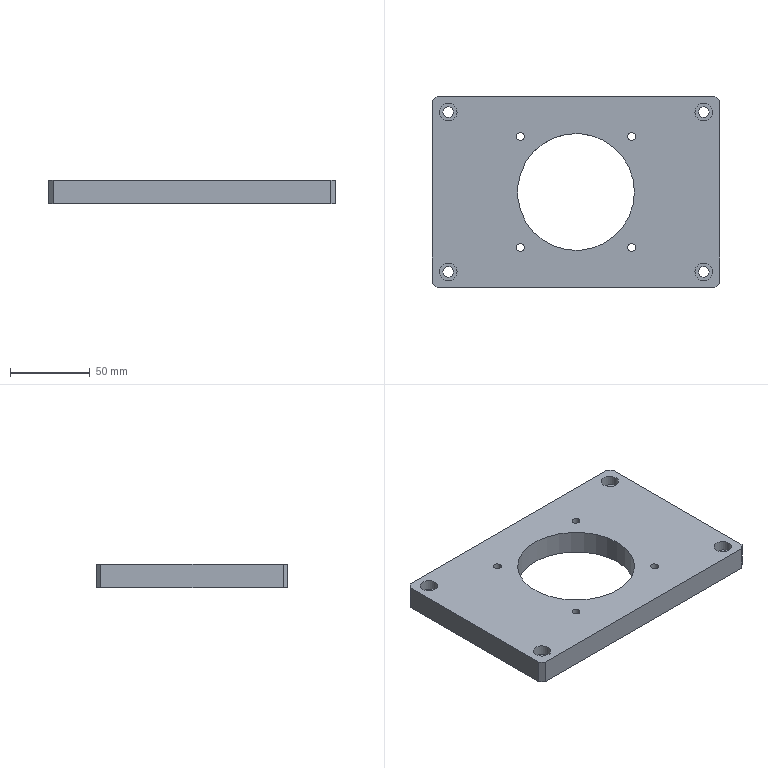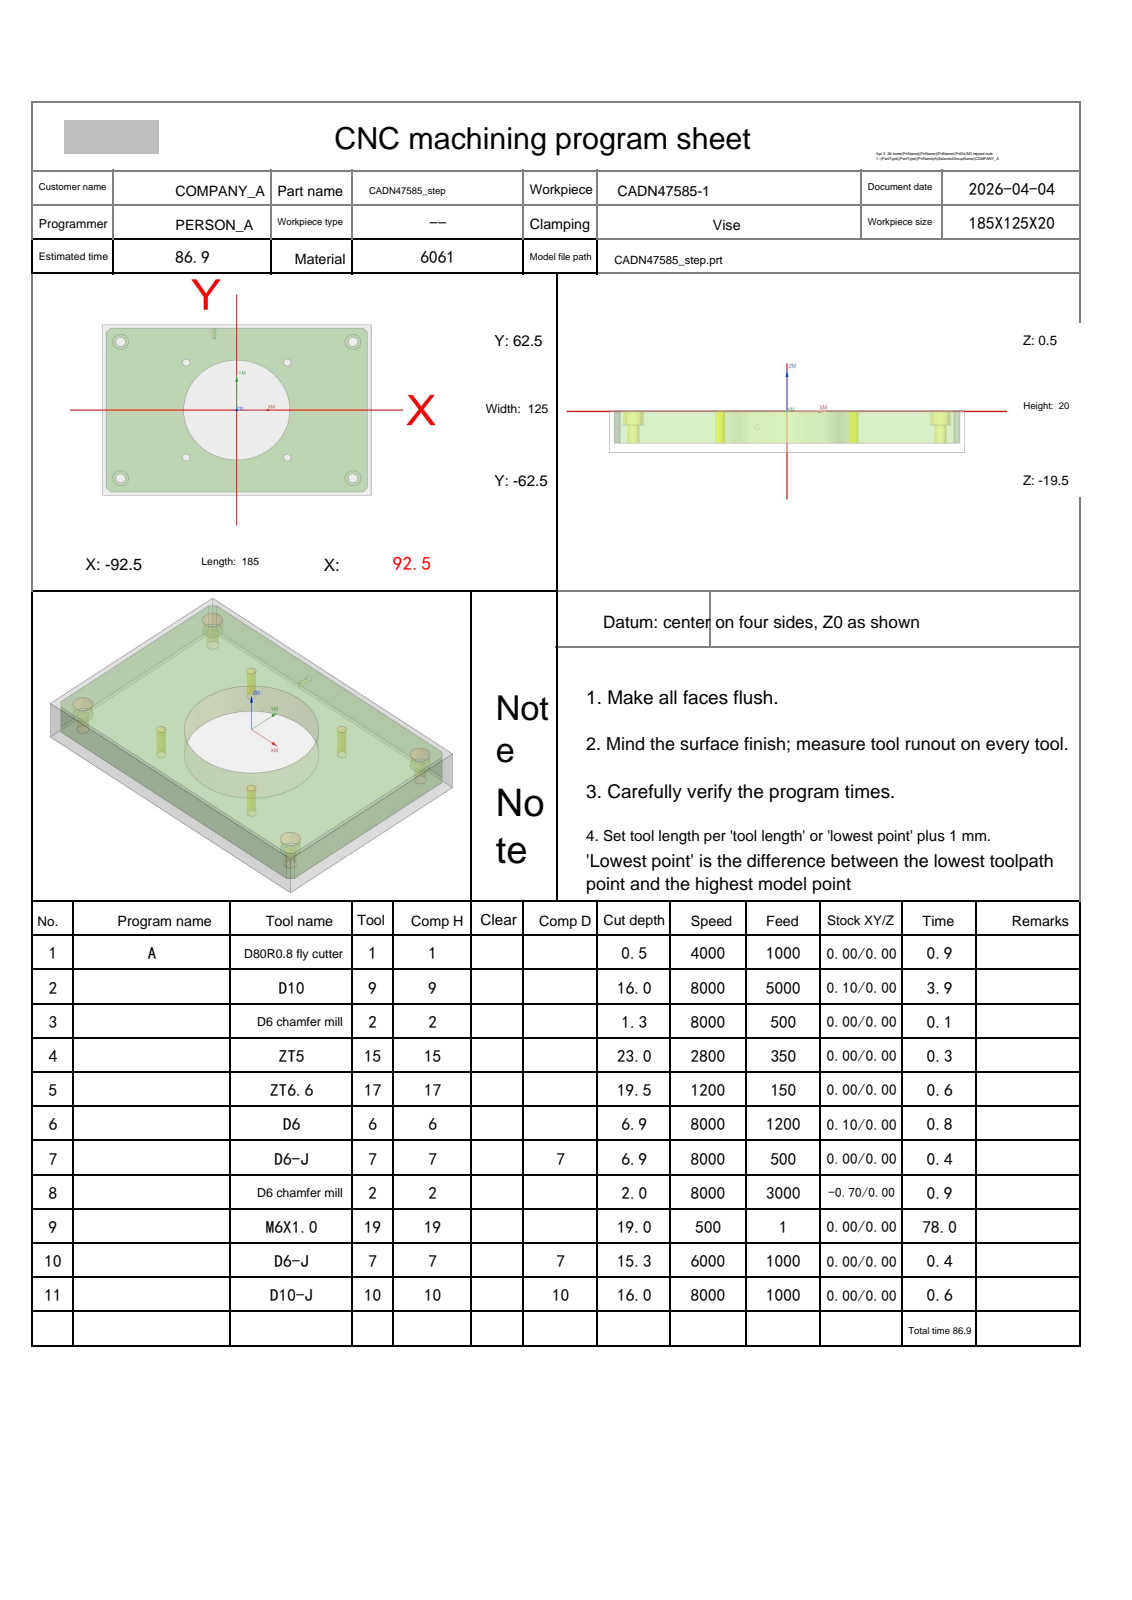NC program | NX | posted by the shop | part box 180 x 120 x 15 mm
Whole program:
%
O0001
(Machine time: 163.22 MIN)
(===Total Tool:9===)
(T1=D80R0.8 fly cutter D=80.  R=0.8  D-  H01 Z=0.    )
(T9=D10     D=10.  R=0.   D-  H09 Z=-15.5 )
(T2=D6 chamfer mill   D=6.   R=0.   D-  H02 Z=-1.5  )
(T15=ZT5    D=5.   DR_a=118 D-  H15 Z=-22.5 )
(T17=ZT6.6  D=6.6  DR_a=118 D-  H17 Z=-18.98)
(T6=D6      D=6.   R=0.   D-  H06 Z=-6.4  )
(T7=D6-J    D=6.   R=0.   D7  H07 Z=-14.8 )
(T19=M6X1.0 D=5.   DR_a=180 D-  H19 Z=-18.5 )
(T10=D10-J  D=10.  R=0.   D10 H10 Z=-15.5 )
G80 G90 G17 G49 G40
G91 G28 Z0
M01
N1 T01 M06
(D80R0.8 fly cutter  D=80. R=0.8 H=01 ce=0.00 di=0.00)
G00 G90 G54 X-135. Y50. M03 S4000
G43 H01 Z20.
M08
Z2.
G01 Z0.0 F1000.
X-130.
X130.
Y0.0
X-130.
Y-50.
X130.
X135.
Z2.
G00 Z20.
G91 G28 Z0.0
M05
M09
G91 G28 Z0.0
M01
N2 T09 M06
(D10  D=10. R=0. H=09 ce=0.10 di=0.00)
G00 G90 G54 X0.0 Y65.1 M03 S8000
G43 H09 Z20.
M08
Z.5
G01 X87. Z.389 F5000.
G02 X90.606 Y63.606 Z.384 I0.0 J-5.1
G01 X93.606 Y60.606 Z.378
G02 X95.1 Y57. Z.373 I-3.606 J-3.606
G01 Y-57. Z.227
G02 X93.606 Y-60.606 Z.222 I-5.1 J0.0
G01 X90.606 Y-63.606 Z.216
G02 X87. Y-65.1 Z.211 I-3.606 J3.606
G01 X-87. Z-.011
G02 X-90.606 Y-63.606 Z-.016 I0.0 J5.1
G01 X-93.606 Y-60.606 Z-.022
G02 X-95.1 Y-57. Z-.027 I3.606 J3.606
G01 Y57. Z-.173
G02 X-93.606 Y60.606 Z-.178 I5.1 J0.0
G01 X-90.606 Y63.606 Z-.184
G02 X-87. Y65.1 Z-.189 I3.606 J-3.606
G01 X87. Z-.411
G02 X90.606 Y63.606 Z-.416 I0.0 J-5.1
G01 X93.606 Y60.606 Z-.422
G02 X95.1 Y57. Z-.427 I-3.606 J-3.606
G01 Y-57. Z-.573
G02 X93.606 Y-60.606 Z-.578 I-5.1 J0.0
G01 X90.606 Y-63.606 Z-.584
G02 X87. Y-65.1 Z-.589 I-3.606 J3.606
G01 X-87. Z-.811
G02 X-90.606 Y-63.606 Z-.816 I0.0 J5.1
G01 X-93.606 Y-60.606 Z-.822
G02 X-95.1 Y-57. Z-.827 I3.606 J3.606
G01 Y57. Z-.973
G02 X-93.606 Y60.606 Z-.978 I5.1 J0.0
G01 X-90.606 Y63.606 Z-.984
G02 X-87. Y65.1 Z-.989 I3.606 J-3.606
G01 X87. Z-1.211
G02 X90.606 Y63.606 Z-1.216 I0.0 J-5.1
G01 X93.606 Y60.606 Z-1.222
G02 X95.1 Y57. Z-1.227 I-3.606 J-3.606
G01 Y-57. Z-1.373
G02 X93.606 Y-60.606 Z-1.378 I-5.1 J0.0
G01 X90.606 Y-63.606 Z-1.384
G02 X87. Y-65.1 Z-1.389 I-3.606 J3.606
G01 X-87. Z-1.611
G02 X-90.606 Y-63.606 Z-1.616 I0.0 J5.1
G01 X-93.606 Y-60.606 Z-1.622
G02 X-95.1 Y-57. Z-1.627 I3.606 J3.606
G01 Y57. Z-1.773
G02 X-93.606 Y60.606 Z-1.778 I5.1 J0.0
G01 X-90.606 Y63.606 Z-1.784
G02 X-87. Y65.1 Z-1.789 I3.606 J-3.606
G01 X87. Z-2.011
G02 X90.606 Y63.606 Z-2.016 I0.0 J-5.1
G01 X93.606 Y60.606 Z-2.022
G02 X95.1 Y57. Z-2.027 I-3.606 J-3.606
G01 Y-57. Z-2.173
G02 X93.606 Y-60.606 Z-2.178 I-5.1 J0.0
G01 X90.606 Y-63.606 Z-2.184
G02 X87. Y-65.1 Z-2.189 I-3.606 J3.606
G01 X-87. Z-2.411
G02 X-90.606 Y-63.606 Z-2.416 I0.0 J5.1
G01 X-93.606 Y-60.606 Z-2.422
G02 X-95.1 Y-57. Z-2.427 I3.606 J3.606
G01 Y57. Z-2.573
G02 X-93.606 Y60.606 Z-2.578 I5.1 J0.0
G01 X-90.606 Y63.606 Z-2.584
G02 X-87. Y65.1 Z-2.589 I3.606 J-3.606
G01 X87. Z-2.811
G02 X90.606 Y63.606 Z-2.816 I0.0 J-5.1
G01 X93.606 Y60.606 Z-2.822
G02 X95.1 Y57. Z-2.827 I-3.606 J-3.606
G01 Y-57. Z-2.973
G02 X93.606 Y-60.606 Z-2.978 I-5.1 J0.0
G01 X90.606 Y-63.606 Z-2.984
G02 X87. Y-65.1 Z-2.989 I-3.606 J3.606
G01 X-87. Z-3.211
G02 X-90.606 Y-63.606 Z-3.216 I0.0 J5.1
G01 X-93.606 Y-60.606 Z-3.222
G02 X-95.1 Y-57. Z-3.227 I3.606 J3.606
G01 Y57. Z-3.373
G02 X-93.606 Y60.606 Z-3.378 I5.1 J0.0
G01 X-90.606 Y63.606 Z-3.384
G02 X-87. Y65.1 Z-3.389 I3.606 J-3.606
G01 X87. Z-3.611
G02 X90.606 Y63.606 Z-3.616 I0.0 J-5.1
G01 X93.606 Y60.606 Z-3.622
G02 X95.1 Y57. Z-3.627 I-3.606 J-3.606
G01 Y-57. Z-3.773
G02 X93.606 Y-60.606 Z-3.778 I-5.1 J0.0
G01 X90.606 Y-63.606 Z-3.784
G02 X87. Y-65.1 Z-3.789 I-3.606 J3.606
G01 X-87. Z-4.011
G02 X-90.606 Y-63.606 Z-4.016 I0.0 J5.1
G01 X-93.606 Y-60.606 Z-4.022
G02 X-95.1 Y-57. Z-4.027 I3.606 J3.606
G01 Y57. Z-4.173
G02 X-93.606 Y60.606 Z-4.178 I5.1 J0.0
G01 X-90.606 Y63.606 Z-4.184
G02 X-87. Y65.1 Z-4.189 I3.606 J-3.606
G01 X87. Z-4.411
G02 X90.606 Y63.606 Z-4.416 I0.0 J-5.1
G01 X93.606 Y60.606 Z-4.422
G02 X95.1 Y57. Z-4.427 I-3.606 J-3.606
G01 Y-57. Z-4.573
G02 X93.606 Y-60.606 Z-4.578 I-5.1 J0.0
G01 X90.606 Y-63.606 Z-4.584
G02 X87. Y-65.1 Z-4.589 I-3.606 J3.606
G01 X-87. Z-4.811
G02 X-90.606 Y-63.606 Z-4.816 I0.0 J5.1
G01 X-93.606 Y-60.606 Z-4.822
G02 X-95.1 Y-57. Z-4.827 I3.606 J3.606
G01 Y57. Z-4.973
G02 X-93.606 Y60.606 Z-4.978 I5.1 J0.0
G01 X-90.606 Y63.606 Z-4.984
G02 X-87. Y65.1 Z-4.989 I3.606 J-3.606
G01 X87. Z-5.211
G02 X90.606 Y63.606 Z-5.216 I0.0 J-5.1
G01 X93.606 Y60.606 Z-5.222
G02 X95.1 Y57. Z-5.227 I-3.606 J-3.606
G01 Y-57. Z-5.373
G02 X93.606 Y-60.606 Z-5.378 I-5.1 J0.0
G01 X90.606 Y-63.606 Z-5.384
G02 X87. Y-65.1 Z-5.389 I-3.606 J3.606
G01 X-87. Z-5.611
G02 X-90.606 Y-63.606 Z-5.616 I0.0 J5.1
G01 X-93.606 Y-60.606 Z-5.622
G02 X-95.1 Y-57. Z-5.627 I3.606 J3.606
G01 Y57. Z-5.773
G02 X-93.606 Y60.606 Z-5.778 I5.1 J0.0
G01 X-90.606 Y63.606 Z-5.784
G02 X-87. Y65.1 Z-5.789 I3.606 J-3.606
G01 X87. Z-6.011
G02 X90.606 Y63.606 Z-6.016 I0.0 J-5.1
G01 X93.606 Y60.606 Z-6.022
G02 X95.1 Y57. Z-6.027 I-3.606 J-3.606
G01 Y-57. Z-6.173
G02 X93.606 Y-60.606 Z-6.178 I-5.1 J0.0
G01 X90.606 Y-63.606 Z-6.184
G02 X87. Y-65.1 Z-6.189 I-3.606 J3.606
G01 X-87. Z-6.411
G02 X-90.606 Y-63.606 Z-6.416 I0.0 J5.1
G01 X-93.606 Y-60.606 Z-6.422
G02 X-95.1 Y-57. Z-6.427 I3.606 J3.606
G01 Y57. Z-6.573
G02 X-93.606 Y60.606 Z-6.578 I5.1 J0.0
G01 X-90.606 Y63.606 Z-6.584
G02 X-87. Y65.1 Z-6.589 I3.606 J-3.606
G01 X87. Z-6.811
G02 X90.606 Y63.606 Z-6.816 I0.0 J-5.1
G01 X93.606 Y60.606 Z-6.822
G02 X95.1 Y57. Z-6.827 I-3.606 J-3.606
G01 Y-57. Z-6.973
G02 X93.606 Y-60.606 Z-6.978 I-5.1 J0.0
G01 X90.606 Y-63.606 Z-6.984
G02 X87. Y-65.1 Z-6.989 I-3.606 J3.606
G01 X-87. Z-7.211
G02 X-90.606 Y-63.606 Z-7.216 I0.0 J5.1
G01 X-93.606 Y-60.606 Z-7.222
G02 X-95.1 Y-57. Z-7.227 I3.606 J3.606
G01 Y57. Z-7.373
G02 X-93.606 Y60.606 Z-7.378 I5.1 J0.0
G01 X-90.606 Y63.606 Z-7.384
G02 X-87. Y65.1 Z-7.389 I3.606 J-3.606
G01 X87. Z-7.611
G02 X90.606 Y63.606 Z-7.616 I0.0 J-5.1
G01 X93.606 Y60.606 Z-7.622
G02 X95.1 Y57. Z-7.627 I-3.606 J-3.606
G01 Y-57. Z-7.773
G02 X93.606 Y-60.606 Z-7.778 I-5.1 J0.0
G01 X90.606 Y-63.606 Z-7.784
G02 X87. Y-65.1 Z-7.789 I-3.606 J3.606
G01 X-87. Z-8.011
G02 X-90.606 Y-63.606 Z-8.016 I0.0 J5.1
G01 X-93.606 Y-60.606 Z-8.022
G02 X-95.1 Y-57. Z-8.027 I3.606 J3.606
G01 Y57. Z-8.173
G02 X-93.606 Y60.606 Z-8.178 I5.1 J0.0
G01 X-90.606 Y63.606 Z-8.184
G02 X-87. Y65.1 Z-8.189 I3.606 J-3.606
G01 X87. Z-8.411
G02 X90.606 Y63.606 Z-8.416 I0.0 J-5.1
G01 X93.606 Y60.606 Z-8.422
G02 X95.1 Y57. Z-8.427 I-3.606 J-3.606
G01 Y-57. Z-8.573
G02 X93.606 Y-60.606 Z-8.578 I-5.1 J0.0
G01 X90.606 Y-63.606 Z-8.584
G02 X87. Y-65.1 Z-8.589 I-3.606 J3.606
G01 X-87. Z-8.811
G02 X-90.606 Y-63.606 Z-8.816 I0.0 J5.1
G01 X-93.606 Y-60.606 Z-8.822
G02 X-95.1 Y-57. Z-8.827 I3.606 J3.606
G01 Y57. Z-8.973
G02 X-93.606 Y60.606 Z-8.978 I5.1 J0.0
G01 X-90.606 Y63.606 Z-8.984
G02 X-87. Y65.1 Z-8.989 I3.606 J-3.606
G01 X87. Z-9.211
G02 X90.606 Y63.606 Z-9.216 I0.0 J-5.1
G01 X93.606 Y60.606 Z-9.222
G02 X95.1 Y57. Z-9.227 I-3.606 J-3.606
G01 Y-57. Z-9.373
G02 X93.606 Y-60.606 Z-9.378 I-5.1 J0.0
G01 X90.606 Y-63.606 Z-9.384
G02 X87. Y-65.1 Z-9.389 I-3.606 J3.606
G01 X-87. Z-9.611
G02 X-90.606 Y-63.606 Z-9.616 I0.0 J5.1
G01 X-93.606 Y-60.606 Z-9.622
G02 X-95.1 Y-57. Z-9.627 I3.606 J3.606
G01 Y57. Z-9.773
G02 X-93.606 Y60.606 Z-9.778 I5.1 J0.0
G01 X-90.606 Y63.606 Z-9.784
G02 X-87. Y65.1 Z-9.789 I3.606 J-3.606
G01 X87. Z-10.011
G02 X90.606 Y63.606 Z-10.016 I0.0 J-5.1
G01 X93.606 Y60.606 Z-10.022
G02 X95.1 Y57. Z-10.027 I-3.606 J-3.606
G01 Y-57. Z-10.173
G02 X93.606 Y-60.606 Z-10.178 I-5.1 J0.0
G01 X90.606 Y-63.606 Z-10.184
G02 X87. Y-65.1 Z-10.189 I-3.606 J3.606
G01 X-87. Z-10.411
G02 X-90.606 Y-63.606 Z-10.416 I0.0 J5.1
G01 X-93.606 Y-60.606 Z-10.422
G02 X-95.1 Y-57. Z-10.427 I3.606 J3.606
G01 Y57. Z-10.573
G02 X-93.606 Y60.606 Z-10.578 I5.1 J0.0
G01 X-90.606 Y63.606 Z-10.584
G02 X-87. Y65.1 Z-10.589 I3.606 J-3.606
G01 X87. Z-10.811
G02 X90.606 Y63.606 Z-10.816 I0.0 J-5.1
G01 X93.606 Y60.606 Z-10.822
G02 X95.1 Y57. Z-10.827 I-3.606 J-3.606
G01 Y-57. Z-10.973
G02 X93.606 Y-60.606 Z-10.978 I-5.1 J0.0
G01 X90.606 Y-63.606 Z-10.984
G02 X87. Y-65.1 Z-10.989 I-3.606 J3.606
G01 X-87. Z-11.211
G02 X-90.606 Y-63.606 Z-11.216 I0.0 J5.1
G01 X-93.606 Y-60.606 Z-11.222
G02 X-95.1 Y-57. Z-11.227 I3.606 J3.606
G01 Y57. Z-11.373
G02 X-93.606 Y60.606 Z-11.378 I5.1 J0.0
G01 X-90.606 Y63.606 Z-11.384
G02 X-87. Y65.1 Z-11.389 I3.606 J-3.606
G01 X87. Z-11.611
G02 X90.606 Y63.606 Z-11.616 I0.0 J-5.1
G01 X93.606 Y60.606 Z-11.622
G02 X95.1 Y57. Z-11.627 I-3.606 J-3.606
G01 Y-57. Z-11.773
G02 X93.606 Y-60.606 Z-11.778 I-5.1 J0.0
G01 X90.606 Y-63.606 Z-11.784
G02 X87. Y-65.1 Z-11.789 I-3.606 J3.606
G01 X-87. Z-12.011
G02 X-90.606 Y-63.606 Z-12.016 I0.0 J5.1
G01 X-93.606 Y-60.606 Z-12.022
G02 X-95.1 Y-57. Z-12.027 I3.606 J3.606
G01 Y57. Z-12.173
G02 X-93.606 Y60.606 Z-12.178 I5.1 J0.0
G01 X-90.606 Y63.606 Z-12.184
G02 X-87. Y65.1 Z-12.189 I3.606 J-3.606
G01 X87. Z-12.411
G02 X90.606 Y63.606 Z-12.416 I0.0 J-5.1
G01 X93.606 Y60.606 Z-12.422
G02 X95.1 Y57. Z-12.427 I-3.606 J-3.606
G01 Y-57. Z-12.573
G02 X93.606 Y-60.606 Z-12.578 I-5.1 J0.0
G01 X90.606 Y-63.606 Z-12.584
G02 X87. Y-65.1 Z-12.589 I-3.606 J3.606
G01 X-87. Z-12.811
G02 X-90.606 Y-63.606 Z-12.816 I0.0 J5.1
G01 X-93.606 Y-60.606 Z-12.822
G02 X-95.1 Y-57. Z-12.827 I3.606 J3.606
G01 Y57. Z-12.973
G02 X-93.606 Y60.606 Z-12.978 I5.1 J0.0
G01 X-90.606 Y63.606 Z-12.984
G02 X-87. Y65.1 Z-12.989 I3.606 J-3.606
G01 X87. Z-13.211
G02 X90.606 Y63.606 Z-13.216 I0.0 J-5.1
G01 X93.606 Y60.606 Z-13.222
G02 X95.1 Y57. Z-13.227 I-3.606 J-3.606
G01 Y-57. Z-13.373
G02 X93.606 Y-60.606 Z-13.378 I-5.1 J0.0
G01 X90.606 Y-63.606 Z-13.384
G02 X87. Y-65.1 Z-13.389 I-3.606 J3.606
G01 X-87. Z-13.611
G02 X-90.606 Y-63.606 Z-13.616 I0.0 J5.1
G01 X-93.606 Y-60.606 Z-13.622
G02 X-95.1 Y-57. Z-13.627 I3.606 J3.606
G01 Y57. Z-13.773
G02 X-93.606 Y60.606 Z-13.778 I5.1 J0.0
G01 X-90.606 Y63.606 Z-13.784
G02 X-87. Y65.1 Z-13.789 I3.606 J-3.606
G01 X87. Z-14.011
G02 X90.606 Y63.606 Z-14.016 I0.0 J-5.1
G01 X93.606 Y60.606 Z-14.022
G02 X95.1 Y57. Z-14.027 I-3.606 J-3.606
G01 Y-57. Z-14.173
G02 X93.606 Y-60.606 Z-14.178 I-5.1 J0.0
G01 X90.606 Y-63.606 Z-14.184
G02 X87. Y-65.1 Z-14.189 I-3.606 J3.606
G01 X-87. Z-14.411
G02 X-90.606 Y-63.606 Z-14.416 I0.0 J5.1
G01 X-93.606 Y-60.606 Z-14.422
G02 X-95.1 Y-57. Z-14.427 I3.606 J3.606
G01 Y57. Z-14.573
G02 X-93.606 Y60.606 Z-14.578 I5.1 J0.0
G01 X-90.606 Y63.606 Z-14.584
G02 X-87. Y65.1 Z-14.589 I3.606 J-3.606
G01 X87. Z-14.811
G02 X90.606 Y63.606 Z-14.816 I0.0 J-5.1
G01 X93.606 Y60.606 Z-14.822
G02 X95.1 Y57. Z-14.827 I-3.606 J-3.606
G01 Y-57. Z-14.973
G02 X93.606 Y-60.606 Z-14.978 I-5.1 J0.0
G01 X90.606 Y-63.606 Z-14.984
G02 X87. Y-65.1 Z-14.989 I-3.606 J3.606
G01 X-87. Z-15.211
G02 X-90.606 Y-63.606 Z-15.216 I0.0 J5.1
G01 X-93.606 Y-60.606 Z-15.222
G02 X-95.1 Y-57. Z-15.227 I3.606 J3.606
G01 Y57. Z-15.373
G02 X-93.606 Y60.606 Z-15.378 I5.1 J0.0
G01 X-90.606 Y63.606 Z-15.384
G02 X-87. Y65.1 Z-15.389 I3.606 J-3.606
G01 X0.0 Z-15.5
X87.
G02 X90.606 Y63.606 I0.0 J-5.1
G01 X93.606 Y60.606
G02 X95.1 Y57. I-3.606 J-3.606
G01 Y-57.
G02 X93.606 Y-60.606 I-5.1 J0.0
G01 X90.606 Y-63.606
G02 X87. Y-65.1 I-3.606 J3.606
G01 X-87.
G02 X-90.606 Y-63.606 I0.0 J5.1
G01 X-93.606 Y-60.606
G02 X-95.1 Y-57. I3.606 J3.606
G01 Y57.
G02 X-93.606 Y60.606 I5.1 J0.0
G01 X-90.606 Y63.606
G02 X-87. Y65.1 I3.606 J-3.606
G01 X0.0
X.5
Z-14.5
G00 Z20.
G00 G90 X17.938 Y25.912 M03 S8000
Z20.
Z1.
G01 X15.119 Y27.669 Z.826 F4000.
X11.87 Y29.21 Z.637
X8.467 Y30.372 Z.449
X4.953 Y31.139 Z.261
X1.375 Y31.5 Z.072
X0.0 Z0.0
G03 X-31.5 Y0.0 Z-.148 I0.0 J-31.5
X0.0 Y-31.5 Z-.296 I31.5 J0.0
X31.5 Y0.0 Z-.444 I0.0 J31.5
X0.0 Y31.5 Z-.592 I-31.5 J0.0
X-31.5 Y0.0 Z-.74 I0.0 J-31.5
X0.0 Y-31.5 Z-.888 I31.5 J0.0
X31.5 Y0.0 Z-1.036 I0.0 J31.5
X0.0 Y31.5 Z-1.184 I-31.5 J0.0
X-31.5 Y0.0 Z-1.332 I0.0 J-31.5
X0.0 Y-31.5 Z-1.48 I31.5 J0.0
X31.5 Y0.0 Z-1.628 I0.0 J31.5
X0.0 Y31.5 Z-1.776 I-31.5 J0.0
X-31.5 Y0.0 Z-1.924 I0.0 J-31.5
X0.0 Y-31.5 Z-2.072 I31.5 J0.0
X31.5 Y0.0 Z-2.22 I0.0 J31.5
X0.0 Y31.5 Z-2.368 I-31.5 J0.0
X-31.5 Y0.0 Z-2.516 I0.0 J-31.5
X0.0 Y-31.5 Z-2.664 I31.5 J0.0
X31.5 Y0.0 Z-2.812 I0.0 J31.5
X0.0 Y31.5 Z-2.96 I-31.5 J0.0
X-31.5 Y0.0 Z-3.108 I0.0 J-31.5
X0.0 Y-31.5 Z-3.256 I31.5 J0.0
X31.5 Y0.0 Z-3.404 I0.0 J31.5
X0.0 Y31.5 Z-3.552 I-31.5 J0.0
X-31.5 Y0.0 Z-3.7 I0.0 J-31.5
X0.0 Y-31.5 Z-3.848 I31.5 J0.0
X31.5 Y0.0 Z-3.996 I0.0 J31.5
X0.0 Y31.5 Z-4.144 I-31.5 J0.0
X-31.5 Y0.0 Z-4.292 I0.0 J-31.5
X0.0 Y-31.5 Z-4.44 I31.5 J0.0
X31.5 Y0.0 Z-4.588 I0.0 J31.5
X0.0 Y31.5 Z-4.736 I-31.5 J0.0
X-31.5 Y0.0 Z-4.884 I0.0 J-31.5
X0.0 Y-31.5 Z-5.032 I31.5 J0.0
X31.5 Y0.0 Z-5.18 I0.0 J31.5
X0.0 Y31.5 Z-5.328 I-31.5 J0.0
X-31.5 Y0.0 Z-5.476 I0.0 J-31.5
X0.0 Y-31.5 Z-5.624 I31.5 J0.0
X31.5 Y0.0 Z-5.772 I0.0 J31.5
X0.0 Y31.5 Z-5.92 I-31.5 J0.0
X-31.5 Y0.0 Z-6.068 I0.0 J-31.5
X0.0 Y-31.5 Z-6.216 I31.5 J0.0
X31.5 Y0.0 Z-6.364 I0.0 J31.5
X0.0 Y31.5 Z-6.512 I-31.5 J0.0
X-31.5 Y0.0 Z-6.66 I0.0 J-31.5
X0.0 Y-31.5 Z-6.808 I31.5 J0.0
X31.5 Y0.0 Z-6.956 I0.0 J31.5
X0.0 Y31.5 Z-7.104 I-31.5 J0.0
X-31.5 Y0.0 Z-7.252 I0.0 J-31.5
X0.0 Y-31.5 Z-7.4 I31.5 J0.0
X31.5 Y0.0 Z-7.548 I0.0 J31.5
X0.0 Y31.5 Z-7.696 I-31.5 J0.0
X-31.5 Y0.0 Z-7.844 I0.0 J-31.5
X0.0 Y-31.5 Z-7.992 I31.5 J0.0
X31.5 Y0.0 Z-8.14 I0.0 J31.5
X0.0 Y31.5 Z-8.288 I-31.5 J0.0
X-31.5 Y0.0 Z-8.436 I0.0 J-31.5
X0.0 Y-31.5 Z-8.584 I31.5 J0.0
X31.5 Y0.0 Z-8.732 I0.0 J31.5
X0.0 Y31.5 Z-8.88 I-31.5 J0.0
X-31.5 Y0.0 Z-9.028 I0.0 J-31.5
X0.0 Y-31.5 Z-9.176 I31.5 J0.0
X31.5 Y0.0 Z-9.324 I0.0 J31.5
X0.0 Y31.5 Z-9.472 I-31.5 J0.0
X-31.5 Y0.0 Z-9.62 I0.0 J-31.5
X0.0 Y-31.5 Z-9.768 I31.5 J0.0
X31.5 Y0.0 Z-9.916 I0.0 J31.5
X0.0 Y31.5 Z-10.064 I-31.5 J0.0
X-31.5 Y0.0 Z-10.212 I0.0 J-31.5
X0.0 Y-31.5 Z-10.36 I31.5 J0.0
X31.5 Y0.0 Z-10.508 I0.0 J31.5
X0.0 Y31.5 Z-10.656 I-31.5 J0.0
X-31.5 Y0.0 Z-10.804 I0.0 J-31.5
X0.0 Y-31.5 Z-10.952 I31.5 J0.0
X31.5 Y0.0 Z-11.1 I0.0 J31.5
X0.0 Y31.5 Z-11.248 I-31.5 J0.0
X-31.5 Y0.0 Z-11.396 I0.0 J-31.5
X0.0 Y-31.5 Z-11.544 I31.5 J0.0
X31.5 Y0.0 Z-11.692 I0.0 J31.5
X0.0 Y31.5 Z-11.84 I-31.5 J0.0
X-31.5 Y0.0 Z-11.988 I0.0 J-31.5
X0.0 Y-31.5 Z-12.136 I31.5 J0.0
X31.5 Y0.0 Z-12.284 I0.0 J31.5
X0.0 Y31.5 Z-12.432 I-31.5 J0.0
X-31.5 Y0.0 Z-12.58 I0.0 J-31.5
X0.0 Y-31.5 Z-12.728 I31.5 J0.0
X31.5 Y0.0 Z-12.876 I0.0 J31.5
X0.0 Y31.5 Z-13.024 I-31.5 J0.0
X-31.5 Y0.0 Z-13.172 I0.0 J-31.5
X0.0 Y-31.5 Z-13.32 I31.5 J0.0
X31.5 Y0.0 Z-13.468 I0.0 J31.5
X0.0 Y31.5 Z-13.616 I-31.5 J0.0
X-31.5 Y0.0 Z-13.764 I0.0 J-31.5
X0.0 Y-31.5 Z-13.912 I31.5 J0.0
X31.5 Y0.0 Z-14.06 I0.0 J31.5
X0.0 Y31.5 Z-14.208 I-31.5 J0.0
X-31.5 Y0.0 Z-14.356 I0.0 J-31.5
X0.0 Y-31.5 Z-14.504 I31.5 J0.0
X31.5 Y0.0 Z-14.652 I0.0 J31.5
X0.0 Y31.5 Z-14.8 I-31.5 J0.0
X-31.5 Y0.0 I0.0 J-31.5
X0.0 Y-31.5 I31.5 J0.0
X31.5 Y0.0 I0.0 J31.5
X0.0 Y31.5 I-31.5 J0.0
X-.4 Y31.497 I0.0 J-31.5
G01 Z-13.8
G00 Z20.
G91 G28 Z0.0
M05
M09
G91 G28 Z0.0
M01
N3 T02 M06
(D6 chamfer mill  D=6. R=0. H=02 ce=0.00 di=0.10)
G00 G90 G54 X80. Y50. M03 S8000
G43 H02 Z20.
M08
G98 G81 X80. Y50. Z-.8 R1. F500.
X34.8 Y34.8
X-34.8
X-80. Y50.
Y-50.
X-34.8 Y-34.8
X34.8
X80. Y-50.
G80
G00 Z20.
G91 G28 Z0.0
M05
M09
G91 G28 Z0.0
M01
N4 T15 M06
(ZT5 D=5. DR_a=118 H=15)
G00 G90 G54 X-34.8 Y34.8 M03 S2800
G43 H15 Z20.
M08
G98 G83 X-34.8 Y34.8 Z-22.502 R1. F350. Q3.
Y-34.8
X34.8
Y34.8
G80
G00 Z20.
G91 G28 Z0.0
M05
M09
G91 G28 Z0.0
M01
N5 T17 M06
(ZT6.6 D=6.6 DR_a=118 H=17)
G00 G90 G54 X-80. Y-50. M03 S1200
G43 H17 Z20.
M08
G98 G83 X-80. Y-50. Z-18.983 R1. F150. Q2.
Y50.
X80.
Y-50.
G80
G00 Z20.
G91 G28 Z0.0
M05
M09
G91 G28 Z0.0
M01
N6 T06 M06
(D6  D=6. R=0. H=06 ce=0.10 di=0.00)
G00 G90 G54 X-80. Y-50. M03 S8000
G43 H06 Z20.
M08
Z.5
G03 X-78.8 Y-51.2 I1.2 J0.0 F1200.
X-77.6 Y-50. I0.0 J1.2
X-77.6 Y-50. Z0.0 I-2.4 J0.0
X-77.6 Y-50. Z-.5 I-2.4 J0.0
X-77.6 Y-50. Z-1. I-2.4 J0.0
X-77.6 Y-50. Z-1.5 I-2.4 J0.0
X-77.6 Y-50. Z-2. I-2.4 J0.0
X-77.6 Y-50. Z-2.5 I-2.4 J0.0
X-77.6 Y-50. Z-3. I-2.4 J0.0
X-77.6 Y-50. Z-3.5 I-2.4 J0.0
X-77.6 Y-50. Z-4. I-2.4 J0.0
X-77.6 Y-50. Z-4.5 I-2.4 J0.0
X-77.6 Y-50. Z-5. I-2.4 J0.0
X-77.6 Y-50. Z-5.5 I-2.4 J0.0
X-77.6 Y-50. Z-6. I-2.4 J0.0
X-79.258 Y-52.283 Z-6.4 I-2.4 J0.0
X-77.6 Y-50. I-.742 J2.283
X-80. Y-47.6 I-2.4 J0.0
X-82.4 Y-50. I0.0 J-2.4
X-80. Y-52.4 I2.4 J0.0
X-79.258 Y-52.283 I0.0 J2.4
X-78.429 Y-51.141 I-.371 J1.141
X-79.629 Y-49.941 I-1.2 J0.0
X-80. Y-50. I0.0 J-1.2
G00 Z20.
Y50.
Z.5
G03 X-78.8 Y48.8 I1.2 J0.0
X-77.6 Y50. I0.0 J1.2
X-77.6 Y50. Z0.0 I-2.4 J0.0
X-77.6 Y50. Z-.5 I-2.4 J0.0
X-77.6 Y50. Z-1. I-2.4 J0.0
X-77.6 Y50. Z-1.5 I-2.4 J0.0
X-77.6 Y50. Z-2. I-2.4 J0.0
X-77.6 Y50. Z-2.5 I-2.4 J0.0
X-77.6 Y50. Z-3. I-2.4 J0.0
X-77.6 Y50. Z-3.5 I-2.4 J0.0
X-77.6 Y50. Z-4. I-2.4 J0.0
X-77.6 Y50. Z-4.5 I-2.4 J0.0
X-77.6 Y50. Z-5. I-2.4 J0.0
X-77.6 Y50. Z-5.5 I-2.4 J0.0
X-77.6 Y50. Z-6. I-2.4 J0.0
X-79.258 Y47.717 Z-6.4 I-2.4 J0.0
X-77.6 Y50. I-.742 J2.283
X-80. Y52.4 I-2.4 J0.0
X-82.4 Y50. I0.0 J-2.4
X-80. Y47.6 I2.4 J0.0
X-79.258 Y47.717 I0.0 J2.4
X-78.429 Y48.859 I-.371 J1.141
X-79.629 Y50.059 I-1.2 J0.0
X-80. Y50. I0.0 J-1.2
G00 Z20.
X80.
Z.5
G03 X81.2 Y48.8 I1.2 J0.0
X82.4 Y50. I0.0 J1.2
X82.4 Y50. Z0.0 I-2.4 J0.0
X82.4 Y50. Z-.5 I-2.4 J0.0
X82.4 Y50. Z-1. I-2.4 J0.0
X82.4 Y50. Z-1.5 I-2.4 J0.0
X82.4 Y50. Z-2. I-2.4 J0.0
X82.4 Y50. Z-2.5 I-2.4 J0.0
X82.4 Y50. Z-3. I-2.4 J0.0
X82.4 Y50. Z-3.5 I-2.4 J0.0
X82.4 Y50. Z-4. I-2.4 J0.0
X82.4 Y50. Z-4.5 I-2.4 J0.0
X82.4 Y50. Z-5. I-2.4 J0.0
X82.4 Y50. Z-5.5 I-2.4 J0.0
X82.4 Y50. Z-6. I-2.4 J0.0
X80.742 Y47.717 Z-6.4 I-2.4 J0.0
X82.4 Y50. I-.742 J2.283
X80. Y52.4 I-2.4 J0.0
X77.6 Y50. I0.0 J-2.4
X80. Y47.6 I2.4 J0.0
X80.742 Y47.717 I0.0 J2.4
X81.571 Y48.859 I-.371 J1.141
X80.371 Y50.059 I-1.2 J0.0
X80. Y50. I0.0 J-1.2
G00 Z20.
Y-50.
Z.5
G03 X81.2 Y-51.2 I1.2 J0.0
X82.4 Y-50. I0.0 J1.2
X82.4 Y-50. Z0.0 I-2.4 J0.0
X82.4 Y-50. Z-.5 I-2.4 J0.0
X82.4 Y-50. Z-1. I-2.4 J0.0
X82.4 Y-50. Z-1.5 I-2.4 J0.0
X82.4 Y-50. Z-2. I-2.4 J0.0
X82.4 Y-50. Z-2.5 I-2.4 J0.0
X82.4 Y-50. Z-3. I-2.4 J0.0
X82.4 Y-50. Z-3.5 I-2.4 J0.0
X82.4 Y-50. Z-4. I-2.4 J0.0
X82.4 Y-50. Z-4.5 I-2.4 J0.0
X82.4 Y-50. Z-5. I-2.4 J0.0
X82.4 Y-50. Z-5.5 I-2.4 J0.0
X82.4 Y-50. Z-6. I-2.4 J0.0
X80.742 Y-52.283 Z-6.4 I-2.4 J0.0
X82.4 Y-50. I-.742 J2.283
X80. Y-47.6 I-2.4 J0.0
X77.6 Y-50. I0.0 J-2.4
X80. Y-52.4 I2.4 J0.0
X80.742 Y-52.283 I0.0 J2.4
X81.571 Y-51.141 I-.371 J1.141
X80.371 Y-49.941 I-1.2 J0.0
X80. Y-50. I0.0 J-1.2
G00 Z20.
G91 G28 Z0.0
M05
M09
G91 G28 Z0.0
M01
N7 T07 M06
(D6-J  D=6. R=0. H=07 ce=0.00 di=0.00)
G00 G90 G54 X-80. Y-50. M03 S8000
G43 H07 Z20.
M08
Z0.0
G41 D07
G01 X-79.968 Y-50.197 F500.
G03 X-78.742 Y-51.242 I1.226 J.197
X-77.5 Y-50. I0.0 J1.242
X-77.5 Y-50. Z-5. I-2.5 J0.0
X-80.468 Y-47.544 Z-6.4 I-2.5 J0.0
X-82.5 Y-50. I.468 J-2.456
X-80. Y-52.5 I2.5 J0.0
X-77.5 Y-50. I0.0 J2.5
X-80. Y-47.5 I-2.5 J0.0
X-80.468 Y-47.544 I0.0 J-2.5
X-81.478 Y-48.764 I.233 J-1.22
X-80.236 Y-50.006 I1.242 J0.0
G01 X-80.2
G40 X-80. Y-50.
G00 Z20.
Y50.
Z0.0
G41 D07
G01 X-79.968 Y49.803
G03 X-78.742 Y48.758 I1.226 J.197
X-77.5 Y50. I0.0 J1.242
X-77.5 Y50. Z-5. I-2.5 J0.0
X-80.468 Y52.456 Z-6.4 I-2.5 J0.0
X-82.5 Y50. I.468 J-2.456
X-80. Y47.5 I2.5 J0.0
X-77.5 Y50. I0.0 J2.5
X-80. Y52.5 I-2.5 J0.0
X-80.468 Y52.456 I0.0 J-2.5
X-81.478 Y51.236 I.233 J-1.22
X-80.236 Y49.994 I1.242 J0.0
G01 X-80.2
G40 X-80. Y50.
G00 Z20.
X80.
Z0.0
G41 D07
G01 X80.032 Y49.803
G03 X81.258 Y48.758 I1.226 J.197
X82.5 Y50. I0.0 J1.242
X82.5 Y50. Z-5. I-2.5 J0.0
X79.532 Y52.456 Z-6.4 I-2.5 J0.0
X77.5 Y50. I.468 J-2.456
X80. Y47.5 I2.5 J0.0
X82.5 Y50. I0.0 J2.5
X80. Y52.5 I-2.5 J0.0
X79.532 Y52.456 I0.0 J-2.5
X78.522 Y51.236 I.233 J-1.22
X79.764 Y49.994 I1.242 J0.0
G01 X79.8
G40 X80. Y50.
G00 Z20.
Y-50.
Z0.0
G41 D07
G01 X80.032 Y-50.197
G03 X81.258 Y-51.242 I1.226 J.197
X82.5 Y-50. I0.0 J1.242
X82.5 Y-50. Z-5. I-2.5 J0.0
X79.532 Y-47.544 Z-6.4 I-2.5 J0.0
X77.5 Y-50. I.468 J-2.456
X80. Y-52.5 I2.5 J0.0
X82.5 Y-50. I0.0 J2.5
X80. Y-47.5 I-2.5 J0.0
X79.532 Y-47.544 I0.0 J-2.5
X78.522 Y-48.764 I.233 J-1.22
X79.764 Y-50.006 I1.242 J0.0
G01 X79.8
G40 X80. Y-50.
G00 Z20.
G91 G28 Z0.0
M05
M09
G91 G28 Z0.0
M01
N8 T02 M06
(D6 chamfer mill  D=6. R=0. H=02 ce=0.00 di=0.00)
G00 G90 G54 X-.25 Y62.128 M03 S8000
G43 H02 Z20.
M08
Z2.099
G01 Z-1.5 F3000.
G03 X-.33 Y61.828 I.52 J-.3
X-.03 Y61.308 I.6 J0.0
G01 X0.0 Y61.3
X87.
X87.254 Y61.275
X87.497 Y61.201
X87.722 Y61.081
X87.919 Y60.919
X90.919 Y57.919
X91.081 Y57.722
X91.201 Y57.497
X91.275 Y57.254
X91.3 Y57.
Y-57.
X91.275 Y-57.254
X91.201 Y-57.497
X91.081 Y-57.722
X90.919 Y-57.919
X87.919 Y-60.919
X87.722 Y-61.081
X87.497 Y-61.201
X87.254 Y-61.275
X87. Y-61.3
X-87.
X-87.254 Y-61.275
X-87.497 Y-61.201
X-87.722 Y-61.081
X-87.919 Y-60.919
X-90.919 Y-57.919
X-91.081 Y-57.722
X-91.201 Y-57.497
X-91.275 Y-57.254
X-91.3 Y-57.
Y57.
X-91.275 Y57.254
X-91.201 Y57.497
X-91.081 Y57.722
X-90.919 Y57.919
X-87.919 Y60.919
X-87.722 Y61.081
X-87.497 Y61.201
X-87.254 Y61.275
X-87. Y61.3
X0.0
X.03 Y61.308
G03 X.33 Y61.828 I-.3 J.52
X.25 Y62.128 I-.6 J0.0
G01 Z2.099
G00 Z20.
X-34.479 Y.269
Z2.116
G01 Z-1.5
G03 X-34.766 Y.343 I-.288 J-.527
X-35.293 Y.03 I0.0 J-.6
G01 X-35.3 Y0.0
G03 X0.0 Y-35.3 I35.3 J0.0
X35.3 Y0.0 I0.0 J35.3
X0.0 Y35.3 I-35.3 J0.0
X-35.3 Y0.0 I0.0 J-35.3
G01 X-35.293 Y-.03
G03 X-34.766 Y-.343 I.527 J.288
X-34.479 Y-.269 I0.0 J.6
G01 Z2.116
G00 Z20.
G00 G90 X34.643 Y35.584 M03 S8000
Z20.
Z-.5
G01 Z-1. F500.
X34.5 Y36.3
G03 X33. Y34.8 I0.0 J-1.5
X34.8 Y33. I1.8 J0.0
X36.6 Y34.8 I0.0 J1.8
X34.8 Y36.6 I-1.8 J0.0
X33. Y34.8 I0.0 J-1.8
X34.5 Y33.3 I1.5 J0.0
G01 X34.643 Y34.016
Z-.5
G00 Z20.
Y-34.016
Z-.5
G01 Z-1.
X34.5 Y-33.3
G03 X33. Y-34.8 I0.0 J-1.5
X34.8 Y-36.6 I1.8 J0.0
X36.6 Y-34.8 I0.0 J1.8
X34.8 Y-33. I-1.8 J0.0
X33. Y-34.8 I0.0 J-1.8
X34.5 Y-36.3 I1.5 J0.0
G01 X34.643 Y-35.584
Z-.5
G00 Z20.
X-34.957 Y-34.016
Z-.5
G01 Z-1.
X-35.1 Y-33.3
G03 X-36.6 Y-34.8 I0.0 J-1.5
X-34.8 Y-36.6 I1.8 J0.0
X-33. Y-34.8 I0.0 J1.8
X-34.8 Y-33. I-1.8 J0.0
X-36.6 Y-34.8 I0.0 J-1.8
X-35.1 Y-36.3 I1.5 J0.0
G01 X-34.957 Y-35.584
Z-.5
G00 Z20.
Y35.584
Z-.5
G01 Z-1.
X-35.1 Y36.3
G03 X-36.6 Y34.8 I0.0 J-1.5
X-34.8 Y33. I1.8 J0.0
X-33. Y34.8 I0.0 J1.8
X-34.8 Y36.6 I-1.8 J0.0
X-36.6 Y34.8 I0.0 J-1.8
X-35.1 Y33.3 I1.5 J0.0
G01 X-34.957 Y34.016
Z-.5
G00 Z20.
G00 G90 X77.991 Y45.643 M03 S8000
Z20.
Z2.5
G01 X78.166 Y45.561 Z2.43 F800.
X78.601 Y45.405 Z2.261
X79.05 Y45.292 Z2.093
X79.507 Y45.222 Z1.925
X79.969 Y45.197 Z1.756
X80.431 Y45.216 Z1.588
X80.89 Y45.28 Z1.419
X81.34 Y45.388 Z1.251
X81.777 Y45.538 Z1.083
X82.198 Y45.73 Z.914
X82.599 Y45.961 Z.746
X82.976 Y46.23 Z.577
X83.325 Y46.534 Z.409
X83.643 Y46.87 Z.241
X83.927 Y47.235 Z.072
X84.175 Y47.625 Z-.096
X84.384 Y48.038 Z-.265
X84.552 Y48.469 Z-.433
X84.679 Y48.914 Z-.601
X84.761 Y49.369 Z-.77
X84.8 Y49.83 Z-.938
Y50. Z-1.
G03 X80. Y54.8 I-4.8 J0.0
X75.2 Y50. I0.0 J-4.8
X80. Y45.2 I4.8 J0.0
X84.8 Y50. I0.0 J4.8
X84.774 Y50.499 I-4.8 J0.0
G01 Z1.5
G00 Z20.
X77.991 Y-54.357
Z2.5
G01 X78.166 Y-54.439 Z2.43
X78.601 Y-54.595 Z2.261
X79.05 Y-54.708 Z2.093
X79.507 Y-54.778 Z1.925
X79.969 Y-54.803 Z1.756
X80.431 Y-54.784 Z1.588
X80.89 Y-54.72 Z1.419
X81.34 Y-54.612 Z1.251
X81.777 Y-54.462 Z1.083
X82.198 Y-54.27 Z.914
X82.599 Y-54.039 Z.746
X82.976 Y-53.77 Z.577
X83.325 Y-53.466 Z.409
X83.643 Y-53.13 Z.241
X83.927 Y-52.765 Z.072
X84.175 Y-52.375 Z-.096
X84.384 Y-51.962 Z-.265
X84.552 Y-51.531 Z-.433
X84.679 Y-51.086 Z-.601
X84.761 Y-50.631 Z-.77
X84.8 Y-50.17 Z-.938
Y-50. Z-1.
G03 X80. Y-45.2 I-4.8 J0.0
X75.2 Y-50. I0.0 J-4.8
X80. Y-54.8 I4.8 J0.0
X84.8 Y-50. I0.0 J4.8
X84.774 Y-49.501 I-4.8 J0.0
G01 Z1.5
G00 Z20.
X-82.009 Y-54.357
Z2.5
G01 X-81.834 Y-54.439 Z2.43
X-81.399 Y-54.595 Z2.261
X-80.95 Y-54.708 Z2.093
X-80.493 Y-54.778 Z1.925
X-80.031 Y-54.803 Z1.756
X-79.569 Y-54.784 Z1.588
X-79.11 Y-54.72 Z1.419
X-78.66 Y-54.612 Z1.251
X-78.223 Y-54.462 Z1.083
X-77.802 Y-54.27 Z.914
X-77.401 Y-54.039 Z.746
X-77.024 Y-53.77 Z.577
X-76.675 Y-53.466 Z.409
X-76.357 Y-53.13 Z.241
X-76.073 Y-52.765 Z.072
X-75.825 Y-52.375 Z-.096
X-75.616 Y-51.962 Z-.265
X-75.448 Y-51.531 Z-.433
X-75.321 Y-51.086 Z-.601
X-75.239 Y-50.631 Z-.77
X-75.2 Y-50.17 Z-.938
Y-50. Z-1.
G03 X-80. Y-45.2 I-4.8 J0.0
X-84.8 Y-50. I0.0 J-4.8
X-80. Y-54.8 I4.8 J0.0
X-75.2 Y-50. I0.0 J4.8
X-75.226 Y-49.501 I-4.8 J0.0
G01 Z1.5
G00 Z20.
X-82.009 Y45.643
Z2.5
G01 X-81.834 Y45.561 Z2.43
X-81.399 Y45.405 Z2.261
X-80.95 Y45.292 Z2.093
X-80.493 Y45.222 Z1.925
X-80.031 Y45.197 Z1.756
X-79.569 Y45.216 Z1.588
X-79.11 Y45.28 Z1.419
X-78.66 Y45.388 Z1.251
X-78.223 Y45.538 Z1.083
X-77.802 Y45.73 Z.914
X-77.401 Y45.961 Z.746
X-77.024 Y46.23 Z.577
X-76.675 Y46.534 Z.409
X-76.357 Y46.87 Z.241
X-76.073 Y47.235 Z.072
X-75.825 Y47.625 Z-.096
X-75.616 Y48.038 Z-.265
X-75.448 Y48.469 Z-.433
X-75.321 Y48.914 Z-.601
X-75.239 Y49.369 Z-.77
X-75.2 Y49.83 Z-.938
Y50. Z-1.
G03 X-80. Y54.8 I-4.8 J0.0
X-84.8 Y50. I0.0 J-4.8
X-80. Y45.2 I4.8 J0.0
X-75.2 Y50. I0.0 J4.8
X-75.226 Y50.499 I-4.8 J0.0
G01 Z1.5
G00 Z20.
G00 G90 X-35.209 Y35.821 M03 S8000
Z20.
Z-.6
G01 Z-1.1 F500.
X-35.4 Y36.3
G03 X-36.9 Y34.8 I0.0 J-1.5
X-34.8 Y32.7 I2.1 J0.0
X-32.7 Y34.8 I0.0 J2.1
X-34.8 Y36.9 I-2.1 J0.0
X-36.9 Y34.8 I0.0 J-2.1
X-35.4 Y33.3 I1.5 J0.0
G01 X-35.209 Y33.779
Z-.6
G00 Z20.
X34.391 Y35.821
Z-.6
G01 Z-1.1
X34.2 Y36.3
G03 X32.7 Y34.8 I0.0 J-1.5
X34.8 Y32.7 I2.1 J0.0
X36.9 Y34.8 I0.0 J2.1
X34.8 Y36.9 I-2.1 J0.0
X32.7 Y34.8 I0.0 J-2.1
X34.2 Y33.3 I1.5 J0.0
G01 X34.391 Y33.779
Z-.6
G00 Z20.
Y-33.779
Z-.6
G01 Z-1.1
X34.2 Y-33.3
G03 X32.7 Y-34.8 I0.0 J-1.5
X34.8 Y-36.9 I2.1 J0.0
X36.9 Y-34.8 I0.0 J2.1
X34.8 Y-32.7 I-2.1 J0.0
X32.7 Y-34.8 I0.0 J-2.1
X34.2 Y-36.3 I1.5 J0.0
G01 X34.391 Y-35.821
Z-.6
G00 Z20.
X-35.209 Y-33.779
Z-.6
G01 Z-1.1
X-35.4 Y-33.3
G03 X-36.9 Y-34.8 I0.0 J-1.5
X-34.8 Y-36.9 I2.1 J0.0
X-32.7 Y-34.8 I0.0 J2.1
X-34.8 Y-32.7 I-2.1 J0.0
X-36.9 Y-34.8 I0.0 J-2.1
X-35.4 Y-36.3 I1.5 J0.0
G01 X-35.209 Y-35.821
Z-.6
G00 Z20.
G91 G28 Z0.0
M05
M09
G91 G28 Z0.0
M01
N9 T19 M06
(M6X1.0 D=5. DR_a=180 H=19)
G00 G90 G54 X-34.8 Y34.8 M03 S500
G43 H19 Z20.
M08
G95
G98 G84 X-34.8 Y34.8 Z-18.5 R1. F1. Q3.
Y-34.8
X34.8
Y34.8
G80
G94
G00 Z20.
G91 G28 Z0.0
M05
M09
G91 G28 Z0.0
M01
N10 T07 M06
(D6-J  D=6. R=0. H=07 ce=0.00 di=0.00)
G00 G90 G54 X-.9 Y-32.488 M03 S6000
G43 H07 Z10.5
M08
Z-5.9
G01 Z-7.4 F1000.
G41 D07
Y-32.7
G03 X0.0 Y-33.6 I.9 J0.0
X33.6 Y0.0 I0.0 J33.6
X0.0 Y33.6 I-33.6 J0.0
X-33.6 Y0.0 I0.0 J-33.6
X0.0 Y-33.6 I33.6 J0.0
X.4 Y-33.598 I0.0 J33.6
X1.289 Y-32.698 I-.011 J.9
G01 Y-32.687
Y-32.675
G40 X1.287 Y-32.475
Z-5.9
G00 X-.9 Y-32.488
Z-13.3
G01 Z-14.8
G41 D07
Y-32.7
G03 X0.0 Y-33.6 I.9 J0.0
X33.6 Y0.0 I0.0 J33.6
X0.0 Y33.6 I-33.6 J0.0
X-33.6 Y0.0 I0.0 J-33.6
X0.0 Y-33.6 I33.6 J0.0
X.4 Y-33.598 I0.0 J33.6
X1.289 Y-32.698 I-.011 J.9
G01 Y-32.687
Y-32.675
G40 X1.287 Y-32.475
Z-13.3
G00 Z10.5
G91 G28 Z0.0
M05
M09
G91 G28 Z0.0
M01
N11 T10 M06
(D10-J  D=10. R=0. H=10 ce=0.00 di=0.00)
G00 G90 G54 X-88.855 Y65.915 M03 S8000
G43 H10 Z20.
M08
Z-15.
G01 Z-15.5 F1000.
G41 D10
X-88.811 Y65.72
G03 X-87.836 Y64.942 I.975 J.221
G01 X-87.696 Y64.951
G02 X-87. Y65. I.696 J-4.951
G01 X87.
G02 X90.536 Y63.536 I0.0 J-5.
G01 X93.536 Y60.536
G02 X95. Y57. I-3.536 J-3.536
G01 Y-57.
G02 X93.536 Y-60.536 I-5. J0.0
G01 X90.536 Y-63.536
G02 X87. Y-65. I-3.536 J3.536
G01 X-87.
G02 X-90.536 Y-63.536 I0.0 J5.
G01 X-93.536 Y-60.536
G02 X-95. Y-57. I3.536 J3.536
G01 Y57.
G02 X-93.536 Y60.536 I5. J0.0
G01 X-90.536 Y63.536
G02 X-87.696 Y64.951 I3.536 J-3.536
X-87.199 Y64.996 I.696 J-4.951
G03 X-86.238 Y65.995 I-.04 J.999
G01 Y66.
G40 X-86.239 Y66.2
Z-15.
G00 Z20.
M05
M09
G91 G28 Z0.0
G91 G28 Y0.0
M30
%